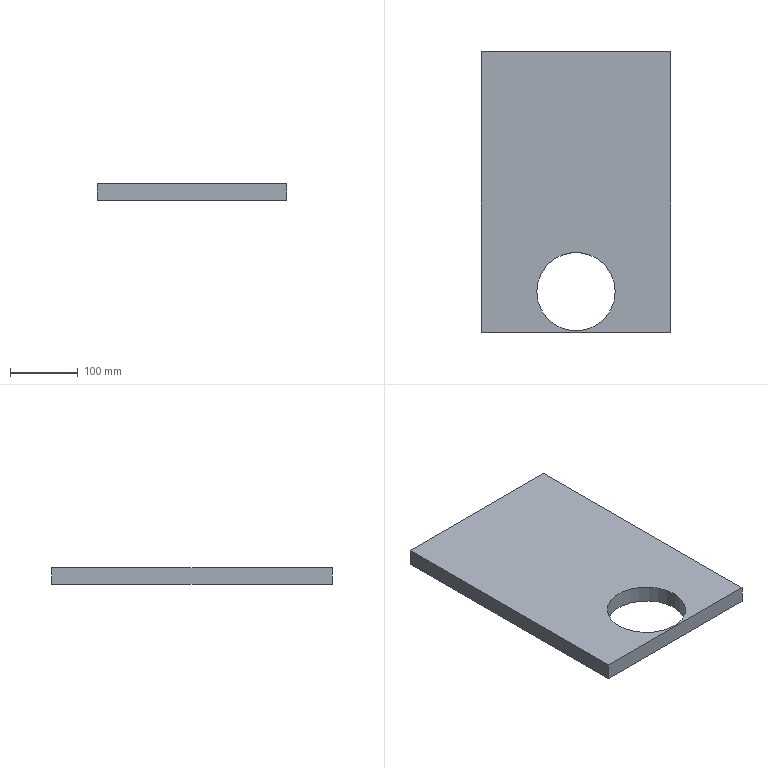Part | SolidWorks | features Extrusion 1 | 1 solid | 8 faces | box 280 x 415 x 25 mm | volume 2640792 mm3 | plane 6 | cylinder 2 | commonest cylinder face diameters 116 x2
STEP:
#1=CARTESIAN_POINT('',(82.,-355.,25.));
#2=VERTEX_POINT('',#1);
#3=CARTESIAN_POINT('',(198.,-355.,25.));
#4=VERTEX_POINT('',#3);
#5=CARTESIAN_POINT('',(140.,-355.,25.));
#6=DIRECTION('',(0.,0.,1.));
#7=DIRECTION('',(1.,0.,0.));
#8=AXIS2_PLACEMENT_3D('',#5,#6,#7);
#9=CIRCLE('',#8,58.);
#10=EDGE_CURVE('',#2,#4,#9,.T.);
#11=ORIENTED_EDGE('',*,*,#10,.T.);
#12=CARTESIAN_POINT('',(198.,-355.,0.));
#13=VERTEX_POINT('',#12);
#14=CARTESIAN_POINT('',(198.,-355.,25.));
#15=DIRECTION('',(0.,0.,-1.));
#16=VECTOR('',#15,1000.);
#17=LINE('',#14,#16);
#18=EDGE_CURVE('',#4,#13,#17,.T.);
#19=ORIENTED_EDGE('',*,*,#18,.T.);
#20=CARTESIAN_POINT('',(82.,-355.,0.));
#21=VERTEX_POINT('',#20);
#22=CARTESIAN_POINT('',(140.,-355.,0.));
#23=DIRECTION('',(0.,0.,1.));
#24=DIRECTION('',(1.,0.,0.));
#25=AXIS2_PLACEMENT_3D('',#22,#23,#24);
#26=CIRCLE('',#25,58.);
#27=EDGE_CURVE('',#21,#13,#26,.T.);
#28=ORIENTED_EDGE('',*,*,#27,.F.);
#29=CARTESIAN_POINT('',(82.,-355.,25.));
#30=DIRECTION('',(0.,0.,-1.));
#31=VECTOR('',#30,1000.);
#32=LINE('',#29,#31);
#33=EDGE_CURVE('',#2,#21,#32,.T.);
#34=ORIENTED_EDGE('',*,*,#33,.F.);
#35=EDGE_LOOP('',(#11,#19,#28,#34));
#36=FACE_OUTER_BOUND('',#35,.T.);
#37=CARTESIAN_POINT('',(140.,-355.,25.));
#38=DIRECTION('',(0.,0.,-1.));
#39=DIRECTION('',(-1.,0.,0.));
#40=AXIS2_PLACEMENT_3D('',#37,#38,#39);
#41=CYLINDRICAL_SURFACE('',#40,58.);
#42=ADVANCED_FACE('',(#36),#41,.F.);
#43=CARTESIAN_POINT('',(0.,0.,25.));
#44=VERTEX_POINT('',#43);
#45=CARTESIAN_POINT('',(0.,-415.,25.));
#46=VERTEX_POINT('',#45);
#47=CARTESIAN_POINT('',(0.,0.,25.));
#48=DIRECTION('',(0.,-1.,0.));
#49=VECTOR('',#48,1000.);
#50=LINE('',#47,#49);
#51=EDGE_CURVE('',#44,#46,#50,.T.);
#52=ORIENTED_EDGE('',*,*,#51,.T.);
#53=CARTESIAN_POINT('',(280.,-415.,25.));
#54=VERTEX_POINT('',#53);
#55=CARTESIAN_POINT('',(0.,-415.,25.));
#56=DIRECTION('',(1.,0.,0.));
#57=VECTOR('',#56,1000.);
#58=LINE('',#55,#57);
#59=EDGE_CURVE('',#46,#54,#58,.T.);
#60=ORIENTED_EDGE('',*,*,#59,.T.);
#61=CARTESIAN_POINT('',(280.,0.,25.));
#62=VERTEX_POINT('',#61);
#63=CARTESIAN_POINT('',(280.,0.,25.));
#64=DIRECTION('',(0.,1.,0.));
#65=VECTOR('',#64,1000.);
#66=LINE('',#63,#65);
#67=EDGE_CURVE('',#54,#62,#66,.T.);
#68=ORIENTED_EDGE('',*,*,#67,.T.);
#69=CARTESIAN_POINT('',(0.,0.,25.));
#70=DIRECTION('',(-1.,0.,0.));
#71=VECTOR('',#70,1000.);
#72=LINE('',#69,#71);
#73=EDGE_CURVE('',#62,#44,#72,.T.);
#74=ORIENTED_EDGE('',*,*,#73,.T.);
#75=EDGE_LOOP('',(#52,#60,#68,#74));
#76=FACE_OUTER_BOUND('',#75,.T.);
#77=ORIENTED_EDGE('',*,*,#10,.F.);
#78=CARTESIAN_POINT('',(140.,-355.,25.));
#79=DIRECTION('',(0.,0.,1.));
#80=DIRECTION('',(1.,0.,0.));
#81=AXIS2_PLACEMENT_3D('',#78,#79,#80);
#82=CIRCLE('',#81,58.);
#83=EDGE_CURVE('',#4,#2,#82,.T.);
#84=ORIENTED_EDGE('',*,*,#83,.F.);
#85=EDGE_LOOP('',(#77,#84));
#86=FACE_BOUND('',#85,.T.);
#87=CARTESIAN_POINT('',(0.,0.,25.));
#88=DIRECTION('',(0.,0.,1.));
#89=DIRECTION('',(1.,0.,0.));
#90=AXIS2_PLACEMENT_3D('',#87,#88,#89);
#91=PLANE('',#90);
#92=ADVANCED_FACE('',(#76,#86),#91,.T.);
#93=CARTESIAN_POINT('',(0.,0.,0.));
#94=VERTEX_POINT('',#93);
#95=CARTESIAN_POINT('',(0.,-415.,0.));
#96=VERTEX_POINT('',#95);
#97=CARTESIAN_POINT('',(0.,0.,0.));
#98=DIRECTION('',(0.,-1.,0.));
#99=VECTOR('',#98,1000.);
#100=LINE('',#97,#99);
#101=EDGE_CURVE('',#94,#96,#100,.T.);
#102=ORIENTED_EDGE('',*,*,#101,.F.);
#103=CARTESIAN_POINT('',(280.,0.,0.));
#104=VERTEX_POINT('',#103);
#105=CARTESIAN_POINT('',(0.,0.,0.));
#106=DIRECTION('',(-1.,0.,0.));
#107=VECTOR('',#106,1000.);
#108=LINE('',#105,#107);
#109=EDGE_CURVE('',#104,#94,#108,.T.);
#110=ORIENTED_EDGE('',*,*,#109,.F.);
#111=CARTESIAN_POINT('',(280.,-415.,0.));
#112=VERTEX_POINT('',#111);
#113=CARTESIAN_POINT('',(280.,0.,0.));
#114=DIRECTION('',(0.,1.,0.));
#115=VECTOR('',#114,1000.);
#116=LINE('',#113,#115);
#117=EDGE_CURVE('',#112,#104,#116,.T.);
#118=ORIENTED_EDGE('',*,*,#117,.F.);
#119=CARTESIAN_POINT('',(0.,-415.,0.));
#120=DIRECTION('',(1.,0.,0.));
#121=VECTOR('',#120,1000.);
#122=LINE('',#119,#121);
#123=EDGE_CURVE('',#96,#112,#122,.T.);
#124=ORIENTED_EDGE('',*,*,#123,.F.);
#125=EDGE_LOOP('',(#102,#110,#118,#124));
#126=FACE_OUTER_BOUND('',#125,.T.);
#127=ORIENTED_EDGE('',*,*,#27,.T.);
#128=CARTESIAN_POINT('',(140.,-355.,0.));
#129=DIRECTION('',(0.,0.,1.));
#130=DIRECTION('',(1.,0.,0.));
#131=AXIS2_PLACEMENT_3D('',#128,#129,#130);
#132=CIRCLE('',#131,58.);
#133=EDGE_CURVE('',#13,#21,#132,.T.);
#134=ORIENTED_EDGE('',*,*,#133,.T.);
#135=EDGE_LOOP('',(#127,#134));
#136=FACE_BOUND('',#135,.T.);
#137=CARTESIAN_POINT('',(0.,0.,0.));
#138=DIRECTION('',(0.,0.,1.));
#139=DIRECTION('',(1.,0.,0.));
#140=AXIS2_PLACEMENT_3D('',#137,#138,#139);
#141=PLANE('',#140);
#142=ADVANCED_FACE('',(#126,#136),#141,.F.);
#143=ORIENTED_EDGE('',*,*,#101,.T.);
#144=CARTESIAN_POINT('',(0.,-415.,25.));
#145=DIRECTION('',(0.,0.,-1.));
#146=VECTOR('',#145,1000.);
#147=LINE('',#144,#146);
#148=EDGE_CURVE('',#46,#96,#147,.T.);
#149=ORIENTED_EDGE('',*,*,#148,.F.);
#150=ORIENTED_EDGE('',*,*,#51,.F.);
#151=CARTESIAN_POINT('',(0.,0.,25.));
#152=DIRECTION('',(0.,0.,-1.));
#153=VECTOR('',#152,1000.);
#154=LINE('',#151,#153);
#155=EDGE_CURVE('',#44,#94,#154,.T.);
#156=ORIENTED_EDGE('',*,*,#155,.T.);
#157=EDGE_LOOP('',(#143,#149,#150,#156));
#158=FACE_OUTER_BOUND('',#157,.T.);
#159=CARTESIAN_POINT('',(0.,0.,25.));
#160=DIRECTION('',(1.,0.,0.));
#161=DIRECTION('',(0.,1.,0.));
#162=AXIS2_PLACEMENT_3D('',#159,#160,#161);
#163=PLANE('',#162);
#164=ADVANCED_FACE('',(#158),#163,.F.);
#165=ORIENTED_EDGE('',*,*,#123,.T.);
#166=CARTESIAN_POINT('',(280.,-415.,25.));
#167=DIRECTION('',(0.,0.,-1.));
#168=VECTOR('',#167,1000.);
#169=LINE('',#166,#168);
#170=EDGE_CURVE('',#54,#112,#169,.T.);
#171=ORIENTED_EDGE('',*,*,#170,.F.);
#172=ORIENTED_EDGE('',*,*,#59,.F.);
#173=ORIENTED_EDGE('',*,*,#148,.T.);
#174=EDGE_LOOP('',(#165,#171,#172,#173));
#175=FACE_OUTER_BOUND('',#174,.T.);
#176=CARTESIAN_POINT('',(0.,-415.,25.));
#177=DIRECTION('',(0.,1.,0.));
#178=DIRECTION('',(0.,0.,1.));
#179=AXIS2_PLACEMENT_3D('',#176,#177,#178);
#180=PLANE('',#179);
#181=ADVANCED_FACE('',(#175),#180,.F.);
#182=ORIENTED_EDGE('',*,*,#117,.T.);
#183=CARTESIAN_POINT('',(280.,0.,25.));
#184=DIRECTION('',(0.,0.,-1.));
#185=VECTOR('',#184,1000.);
#186=LINE('',#183,#185);
#187=EDGE_CURVE('',#62,#104,#186,.T.);
#188=ORIENTED_EDGE('',*,*,#187,.F.);
#189=ORIENTED_EDGE('',*,*,#67,.F.);
#190=ORIENTED_EDGE('',*,*,#170,.T.);
#191=EDGE_LOOP('',(#182,#188,#189,#190));
#192=FACE_OUTER_BOUND('',#191,.T.);
#193=CARTESIAN_POINT('',(280.,0.,25.));
#194=DIRECTION('',(-1.,0.,0.));
#195=DIRECTION('',(0.,-1.,0.));
#196=AXIS2_PLACEMENT_3D('',#193,#194,#195);
#197=PLANE('',#196);
#198=ADVANCED_FACE('',(#192),#197,.F.);
#199=ORIENTED_EDGE('',*,*,#109,.T.);
#200=ORIENTED_EDGE('',*,*,#155,.F.);
#201=ORIENTED_EDGE('',*,*,#73,.F.);
#202=ORIENTED_EDGE('',*,*,#187,.T.);
#203=EDGE_LOOP('',(#199,#200,#201,#202));
#204=FACE_OUTER_BOUND('',#203,.T.);
#205=CARTESIAN_POINT('',(0.,0.,25.));
#206=DIRECTION('',(0.,-1.,0.));
#207=DIRECTION('',(0.,0.,-1.));
#208=AXIS2_PLACEMENT_3D('',#205,#206,#207);
#209=PLANE('',#208);
#210=ADVANCED_FACE('',(#204),#209,.F.);
#211=ORIENTED_EDGE('',*,*,#18,.F.);
#212=ORIENTED_EDGE('',*,*,#83,.T.);
#213=ORIENTED_EDGE('',*,*,#33,.T.);
#214=ORIENTED_EDGE('',*,*,#133,.F.);
#215=EDGE_LOOP('',(#211,#212,#213,#214));
#216=FACE_OUTER_BOUND('',#215,.T.);
#217=CARTESIAN_POINT('',(140.,-355.,25.));
#218=DIRECTION('',(0.,0.,-1.));
#219=DIRECTION('',(-1.,0.,0.));
#220=AXIS2_PLACEMENT_3D('',#217,#218,#219);
#221=CYLINDRICAL_SURFACE('',#220,58.);
#222=ADVANCED_FACE('',(#216),#221,.F.);
#223=CLOSED_SHELL('',(#42,#92,#142,#164,#181,#198,#210,#222));
#224=MANIFOLD_SOLID_BREP('',#223);
#225=CARTESIAN_POINT('',(0.,0.,0.));
#226=DIRECTION('',(0.,0.,1.));
#227=DIRECTION('',(1.,0.,0.));
#228=AXIS2_PLACEMENT_3D('',#225,#226,#227);
#229=(LENGTH_UNIT()NAMED_UNIT(*)SI_UNIT(.MILLI.,.METRE.));
#230=UNCERTAINTY_MEASURE_WITH_UNIT(LENGTH_MEASURE(0.00001),#229,'','');
#231=(NAMED_UNIT(*)PLANE_ANGLE_UNIT()SI_UNIT($,.RADIAN.));
#232=(NAMED_UNIT(*)SI_UNIT($,.STERADIAN.)SOLID_ANGLE_UNIT());
#233=(GEOMETRIC_REPRESENTATION_CONTEXT(3)GLOBAL_UNCERTAINTY_ASSIGNED_CONTEXT((#230))GLOBAL_UNIT_ASSIGNED_CONTEXT((#229,#231,#232))REPRESENTATION_CONTEXT('',''));
#234=ADVANCED_BREP_SHAPE_REPRESENTATION('',(#224,#228),#233);